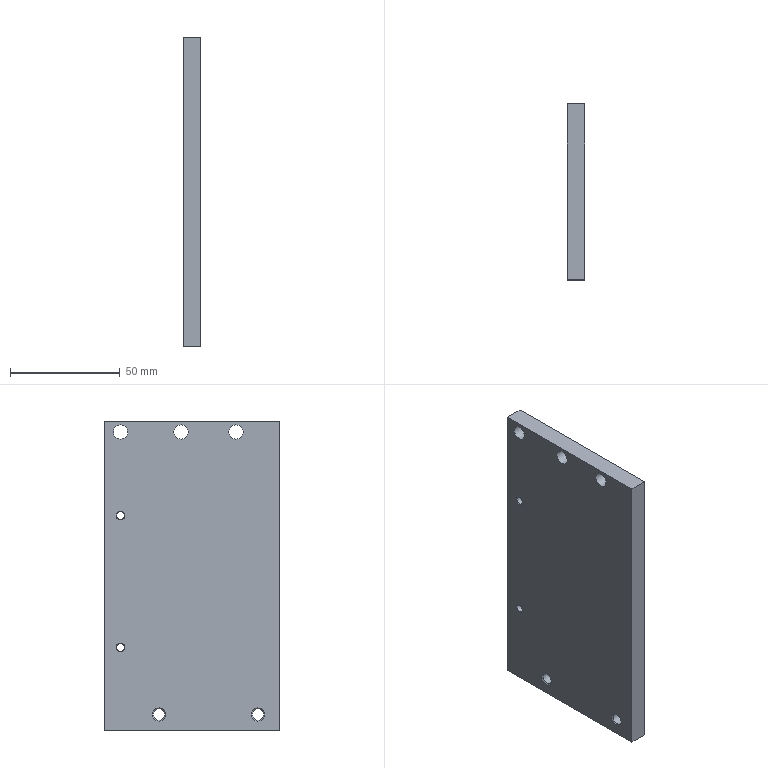Part | NX | features SIMPLE HOLE 7, DATUM_CSYS 5, SKETCH 4, SYMBOLIC_THREAD 4, HOLE PACKAGE 3, EXTRUDE 1 | 1 solid | 21 faces | box 8 x 80 x 141 mm | volume 88943 mm3 | cone 8 | cylinder 7 | plane 6 | commonest cylinder face diameters 6.5 x3 3.5 x2 5.2 x2
STEP:
#1=CARTESIAN_POINT('',(0.,-40.,70.5));
#2=VERTEX_POINT('',#1);
#3=CARTESIAN_POINT('',(0.,-40.,-70.5));
#4=VERTEX_POINT('',#3);
#5=CARTESIAN_POINT('',(0.,-40.,70.5));
#6=DIRECTION('',(0.,0.,-1.));
#7=VECTOR('',#6,1000.);
#8=LINE('',#5,#7);
#9=EDGE_CURVE('',#2,#4,#8,.T.);
#10=ORIENTED_EDGE('',*,*,#9,.T.);
#11=CARTESIAN_POINT('',(8.,-40.,-70.5));
#12=VERTEX_POINT('',#11);
#13=CARTESIAN_POINT('',(8.,-40.,-70.5));
#14=DIRECTION('',(-1.,0.,0.));
#15=VECTOR('',#14,1000.);
#16=LINE('',#13,#15);
#17=EDGE_CURVE('',#12,#4,#16,.T.);
#18=ORIENTED_EDGE('',*,*,#17,.F.);
#19=CARTESIAN_POINT('',(8.,-40.,70.5));
#20=VERTEX_POINT('',#19);
#21=CARTESIAN_POINT('',(8.,-40.,70.5));
#22=DIRECTION('',(0.,0.,-1.));
#23=VECTOR('',#22,1000.);
#24=LINE('',#21,#23);
#25=EDGE_CURVE('',#20,#12,#24,.T.);
#26=ORIENTED_EDGE('',*,*,#25,.F.);
#27=CARTESIAN_POINT('',(8.,-40.,70.5));
#28=DIRECTION('',(-1.,0.,0.));
#29=VECTOR('',#28,1000.);
#30=LINE('',#27,#29);
#31=EDGE_CURVE('',#20,#2,#30,.T.);
#32=ORIENTED_EDGE('',*,*,#31,.T.);
#33=EDGE_LOOP('',(#10,#18,#26,#32));
#34=FACE_BOUND('',#33,.T.);
#35=CARTESIAN_POINT('',(8.,-40.,70.5));
#36=DIRECTION('',(0.,1.,0.));
#37=DIRECTION('',(0.,0.,1.));
#38=AXIS2_PLACEMENT_3D('',#35,#36,#37);
#39=PLANE('',#38);
#40=ADVANCED_FACE('',(#34),#39,.F.);
#41=CARTESIAN_POINT('',(0.,40.,-70.5));
#42=VERTEX_POINT('',#41);
#43=CARTESIAN_POINT('',(0.,-40.,-70.5));
#44=DIRECTION('',(0.,1.,0.));
#45=VECTOR('',#44,1000.);
#46=LINE('',#43,#45);
#47=EDGE_CURVE('',#4,#42,#46,.T.);
#48=ORIENTED_EDGE('',*,*,#47,.T.);
#49=CARTESIAN_POINT('',(8.,40.,-70.5));
#50=VERTEX_POINT('',#49);
#51=CARTESIAN_POINT('',(8.,40.,-70.5));
#52=DIRECTION('',(-1.,0.,0.));
#53=VECTOR('',#52,1000.);
#54=LINE('',#51,#53);
#55=EDGE_CURVE('',#50,#42,#54,.T.);
#56=ORIENTED_EDGE('',*,*,#55,.F.);
#57=CARTESIAN_POINT('',(8.,-40.,-70.5));
#58=DIRECTION('',(0.,1.,0.));
#59=VECTOR('',#58,1000.);
#60=LINE('',#57,#59);
#61=EDGE_CURVE('',#12,#50,#60,.T.);
#62=ORIENTED_EDGE('',*,*,#61,.F.);
#63=ORIENTED_EDGE('',*,*,#17,.T.);
#64=EDGE_LOOP('',(#48,#56,#62,#63));
#65=FACE_BOUND('',#64,.T.);
#66=CARTESIAN_POINT('',(8.,-40.,-70.5));
#67=DIRECTION('',(0.,0.,1.));
#68=DIRECTION('',(1.,0.,0.));
#69=AXIS2_PLACEMENT_3D('',#66,#67,#68);
#70=PLANE('',#69);
#71=ADVANCED_FACE('',(#65),#70,.F.);
#72=CARTESIAN_POINT('',(0.,40.,70.5));
#73=VERTEX_POINT('',#72);
#74=CARTESIAN_POINT('',(0.,40.,-70.5));
#75=DIRECTION('',(0.,0.,1.));
#76=VECTOR('',#75,1000.);
#77=LINE('',#74,#76);
#78=EDGE_CURVE('',#42,#73,#77,.T.);
#79=ORIENTED_EDGE('',*,*,#78,.T.);
#80=CARTESIAN_POINT('',(8.,40.,70.5));
#81=VERTEX_POINT('',#80);
#82=CARTESIAN_POINT('',(8.,40.,70.5));
#83=DIRECTION('',(-1.,0.,0.));
#84=VECTOR('',#83,1000.);
#85=LINE('',#82,#84);
#86=EDGE_CURVE('',#81,#73,#85,.T.);
#87=ORIENTED_EDGE('',*,*,#86,.F.);
#88=CARTESIAN_POINT('',(8.,40.,-70.5));
#89=DIRECTION('',(0.,0.,1.));
#90=VECTOR('',#89,1000.);
#91=LINE('',#88,#90);
#92=EDGE_CURVE('',#50,#81,#91,.T.);
#93=ORIENTED_EDGE('',*,*,#92,.F.);
#94=ORIENTED_EDGE('',*,*,#55,.T.);
#95=EDGE_LOOP('',(#79,#87,#93,#94));
#96=FACE_BOUND('',#95,.T.);
#97=CARTESIAN_POINT('',(8.,40.,-70.5));
#98=DIRECTION('',(0.,-1.,0.));
#99=DIRECTION('',(0.,0.,-1.));
#100=AXIS2_PLACEMENT_3D('',#97,#98,#99);
#101=PLANE('',#100);
#102=ADVANCED_FACE('',(#96),#101,.F.);
#103=CARTESIAN_POINT('',(0.,40.,70.5));
#104=DIRECTION('',(0.,-1.,0.));
#105=VECTOR('',#104,1000.);
#106=LINE('',#103,#105);
#107=EDGE_CURVE('',#73,#2,#106,.T.);
#108=ORIENTED_EDGE('',*,*,#107,.T.);
#109=ORIENTED_EDGE('',*,*,#31,.F.);
#110=CARTESIAN_POINT('',(8.,40.,70.5));
#111=DIRECTION('',(0.,-1.,0.));
#112=VECTOR('',#111,1000.);
#113=LINE('',#110,#112);
#114=EDGE_CURVE('',#81,#20,#113,.T.);
#115=ORIENTED_EDGE('',*,*,#114,.F.);
#116=ORIENTED_EDGE('',*,*,#86,.T.);
#117=EDGE_LOOP('',(#108,#109,#115,#116));
#118=FACE_BOUND('',#117,.T.);
#119=CARTESIAN_POINT('',(8.,40.,70.5));
#120=DIRECTION('',(0.,0.,-1.));
#121=DIRECTION('',(-1.,0.,0.));
#122=AXIS2_PLACEMENT_3D('',#119,#120,#121);
#123=PLANE('',#122);
#124=ADVANCED_FACE('',(#118),#123,.F.);
#125=CARTESIAN_POINT('',(8.,32.5,62.25));
#126=VERTEX_POINT('',#125);
#127=CARTESIAN_POINT('',(8.,32.5,65.5));
#128=DIRECTION('',(1.,0.,0.));
#129=DIRECTION('',(0.,0.,-1.));
#130=AXIS2_PLACEMENT_3D('',#127,#128,#129);
#131=CIRCLE('',#130,3.25);
#132=EDGE_CURVE('',#126,#126,#131,.T.);
#133=ORIENTED_EDGE('',*,*,#132,.F.);
#134=EDGE_LOOP('',(#133));
#135=FACE_BOUND('',#134,.T.);
#136=CARTESIAN_POINT('',(8.,5.,62.25));
#137=VERTEX_POINT('',#136);
#138=CARTESIAN_POINT('',(8.,5.,65.5));
#139=DIRECTION('',(1.,0.,0.));
#140=DIRECTION('',(0.,0.,-1.));
#141=AXIS2_PLACEMENT_3D('',#138,#139,#140);
#142=CIRCLE('',#141,3.25);
#143=EDGE_CURVE('',#137,#137,#142,.T.);
#144=ORIENTED_EDGE('',*,*,#143,.F.);
#145=EDGE_LOOP('',(#144));
#146=FACE_BOUND('',#145,.T.);
#147=CARTESIAN_POINT('',(8.,-20.,62.25));
#148=VERTEX_POINT('',#147);
#149=CARTESIAN_POINT('',(8.,-20.,65.5));
#150=DIRECTION('',(1.,0.,0.));
#151=DIRECTION('',(0.,0.,-1.));
#152=AXIS2_PLACEMENT_3D('',#149,#150,#151);
#153=CIRCLE('',#152,3.25);
#154=EDGE_CURVE('',#148,#148,#153,.T.);
#155=ORIENTED_EDGE('',*,*,#154,.F.);
#156=EDGE_LOOP('',(#155));
#157=FACE_BOUND('',#156,.T.);
#158=CARTESIAN_POINT('',(8.,15.,-66.));
#159=VERTEX_POINT('',#158);
#160=CARTESIAN_POINT('',(8.,15.,-63.));
#161=DIRECTION('',(1.,0.,0.));
#162=DIRECTION('',(0.,0.,-1.));
#163=AXIS2_PLACEMENT_3D('',#160,#161,#162);
#164=CIRCLE('',#163,3.);
#165=EDGE_CURVE('',#159,#159,#164,.F.);
#166=ORIENTED_EDGE('',*,*,#165,.T.);
#167=EDGE_LOOP('',(#166));
#168=FACE_BOUND('',#167,.T.);
#169=CARTESIAN_POINT('',(8.,-30.,-66.));
#170=VERTEX_POINT('',#169);
#171=CARTESIAN_POINT('',(8.,-30.,-63.));
#172=DIRECTION('',(1.,0.,0.));
#173=DIRECTION('',(0.,0.,-1.));
#174=AXIS2_PLACEMENT_3D('',#171,#172,#173);
#175=CIRCLE('',#174,3.);
#176=EDGE_CURVE('',#170,#170,#175,.F.);
#177=ORIENTED_EDGE('',*,*,#176,.T.);
#178=EDGE_LOOP('',(#177));
#179=FACE_BOUND('',#178,.T.);
#180=CARTESIAN_POINT('',(8.,32.5,25.5));
#181=VERTEX_POINT('',#180);
#182=CARTESIAN_POINT('',(8.,32.5,27.5));
#183=DIRECTION('',(1.,0.,0.));
#184=DIRECTION('',(0.,0.,-1.));
#185=AXIS2_PLACEMENT_3D('',#182,#183,#184);
#186=CIRCLE('',#185,2.);
#187=EDGE_CURVE('',#181,#181,#186,.F.);
#188=ORIENTED_EDGE('',*,*,#187,.T.);
#189=EDGE_LOOP('',(#188));
#190=FACE_BOUND('',#189,.T.);
#191=CARTESIAN_POINT('',(8.,32.5,-34.5));
#192=VERTEX_POINT('',#191);
#193=CARTESIAN_POINT('',(8.,32.5,-32.5));
#194=DIRECTION('',(1.,0.,0.));
#195=DIRECTION('',(0.,0.,-1.));
#196=AXIS2_PLACEMENT_3D('',#193,#194,#195);
#197=CIRCLE('',#196,2.);
#198=EDGE_CURVE('',#192,#192,#197,.F.);
#199=ORIENTED_EDGE('',*,*,#198,.T.);
#200=EDGE_LOOP('',(#199));
#201=FACE_BOUND('',#200,.T.);
#202=ORIENTED_EDGE('',*,*,#25,.T.);
#203=ORIENTED_EDGE('',*,*,#61,.T.);
#204=ORIENTED_EDGE('',*,*,#92,.T.);
#205=ORIENTED_EDGE('',*,*,#114,.T.);
#206=EDGE_LOOP('',(#202,#203,#204,#205));
#207=FACE_BOUND('',#206,.T.);
#208=CARTESIAN_POINT('',(8.,0.,0.));
#209=DIRECTION('',(1.,0.,0.));
#210=DIRECTION('',(0.,0.,-1.));
#211=AXIS2_PLACEMENT_3D('',#208,#209,#210);
#212=PLANE('',#211);
#213=ADVANCED_FACE('',(#135,#146,#157,#168,#179,#190,#201,#207),#212,.T.);
#214=CARTESIAN_POINT('',(0.,32.5,62.25));
#215=VERTEX_POINT('',#214);
#216=CARTESIAN_POINT('',(0.,32.5,65.5));
#217=DIRECTION('',(1.,0.,0.));
#218=DIRECTION('',(0.,0.,-1.));
#219=AXIS2_PLACEMENT_3D('',#216,#217,#218);
#220=CIRCLE('',#219,3.25);
#221=EDGE_CURVE('',#215,#215,#220,.T.);
#222=ORIENTED_EDGE('',*,*,#221,.T.);
#223=EDGE_LOOP('',(#222));
#224=FACE_BOUND('',#223,.T.);
#225=CARTESIAN_POINT('',(0.,5.,62.25));
#226=VERTEX_POINT('',#225);
#227=CARTESIAN_POINT('',(0.,5.,65.5));
#228=DIRECTION('',(1.,0.,0.));
#229=DIRECTION('',(0.,0.,-1.));
#230=AXIS2_PLACEMENT_3D('',#227,#228,#229);
#231=CIRCLE('',#230,3.25);
#232=EDGE_CURVE('',#226,#226,#231,.T.);
#233=ORIENTED_EDGE('',*,*,#232,.T.);
#234=EDGE_LOOP('',(#233));
#235=FACE_BOUND('',#234,.T.);
#236=CARTESIAN_POINT('',(0.,-20.,62.25));
#237=VERTEX_POINT('',#236);
#238=CARTESIAN_POINT('',(0.,-20.,65.5));
#239=DIRECTION('',(1.,0.,0.));
#240=DIRECTION('',(0.,0.,-1.));
#241=AXIS2_PLACEMENT_3D('',#238,#239,#240);
#242=CIRCLE('',#241,3.25);
#243=EDGE_CURVE('',#237,#237,#242,.T.);
#244=ORIENTED_EDGE('',*,*,#243,.T.);
#245=EDGE_LOOP('',(#244));
#246=FACE_BOUND('',#245,.T.);
#247=CARTESIAN_POINT('',(0.,15.,-66.));
#248=VERTEX_POINT('',#247);
#249=CARTESIAN_POINT('',(0.,15.,-63.));
#250=DIRECTION('',(1.,0.,0.));
#251=DIRECTION('',(0.,0.,-1.));
#252=AXIS2_PLACEMENT_3D('',#249,#250,#251);
#253=CIRCLE('',#252,3.);
#254=EDGE_CURVE('',#248,#248,#253,.T.);
#255=ORIENTED_EDGE('',*,*,#254,.T.);
#256=EDGE_LOOP('',(#255));
#257=FACE_BOUND('',#256,.T.);
#258=CARTESIAN_POINT('',(0.,-30.,-66.));
#259=VERTEX_POINT('',#258);
#260=CARTESIAN_POINT('',(0.,-30.,-63.));
#261=DIRECTION('',(1.,0.,0.));
#262=DIRECTION('',(0.,0.,-1.));
#263=AXIS2_PLACEMENT_3D('',#260,#261,#262);
#264=CIRCLE('',#263,3.);
#265=EDGE_CURVE('',#259,#259,#264,.T.);
#266=ORIENTED_EDGE('',*,*,#265,.T.);
#267=EDGE_LOOP('',(#266));
#268=FACE_BOUND('',#267,.T.);
#269=CARTESIAN_POINT('',(0.,32.5,25.5));
#270=VERTEX_POINT('',#269);
#271=CARTESIAN_POINT('',(0.,32.5,27.5));
#272=DIRECTION('',(1.,0.,0.));
#273=DIRECTION('',(0.,0.,-1.));
#274=AXIS2_PLACEMENT_3D('',#271,#272,#273);
#275=CIRCLE('',#274,2.);
#276=EDGE_CURVE('',#270,#270,#275,.T.);
#277=ORIENTED_EDGE('',*,*,#276,.T.);
#278=EDGE_LOOP('',(#277));
#279=FACE_BOUND('',#278,.T.);
#280=CARTESIAN_POINT('',(0.,32.5,-34.5));
#281=VERTEX_POINT('',#280);
#282=CARTESIAN_POINT('',(0.,32.5,-32.5));
#283=DIRECTION('',(1.,0.,0.));
#284=DIRECTION('',(0.,0.,-1.));
#285=AXIS2_PLACEMENT_3D('',#282,#283,#284);
#286=CIRCLE('',#285,2.);
#287=EDGE_CURVE('',#281,#281,#286,.T.);
#288=ORIENTED_EDGE('',*,*,#287,.T.);
#289=EDGE_LOOP('',(#288));
#290=FACE_BOUND('',#289,.T.);
#291=ORIENTED_EDGE('',*,*,#9,.F.);
#292=ORIENTED_EDGE('',*,*,#107,.F.);
#293=ORIENTED_EDGE('',*,*,#78,.F.);
#294=ORIENTED_EDGE('',*,*,#47,.F.);
#295=EDGE_LOOP('',(#291,#292,#293,#294));
#296=FACE_BOUND('',#295,.T.);
#297=CARTESIAN_POINT('',(0.,0.,0.));
#298=DIRECTION('',(1.,0.,0.));
#299=DIRECTION('',(0.,0.,-1.));
#300=AXIS2_PLACEMENT_3D('',#297,#298,#299);
#301=PLANE('',#300);
#302=ADVANCED_FACE('',(#224,#235,#246,#257,#268,#279,#290,#296),#301,.F.);
#303=CARTESIAN_POINT('',(0.25,32.5,-34.25));
#304=VERTEX_POINT('',#303);
#305=CARTESIAN_POINT('',(0.25,32.5,-32.5));
#306=DIRECTION('',(1.,0.,0.));
#307=DIRECTION('',(0.,0.,-1.));
#308=AXIS2_PLACEMENT_3D('',#305,#306,#307);
#309=CIRCLE('',#308,1.75);
#310=EDGE_CURVE('',#304,#304,#309,.F.);
#311=ORIENTED_EDGE('',*,*,#310,.T.);
#312=EDGE_LOOP('',(#311));
#313=FACE_BOUND('',#312,.T.);
#314=CARTESIAN_POINT('',(7.75,32.5,-34.25));
#315=VERTEX_POINT('',#314);
#316=CARTESIAN_POINT('',(7.75,32.5,-32.5));
#317=DIRECTION('',(1.,0.,0.));
#318=DIRECTION('',(0.,0.,-1.));
#319=AXIS2_PLACEMENT_3D('',#316,#317,#318);
#320=CIRCLE('',#319,1.75);
#321=EDGE_CURVE('',#315,#315,#320,.T.);
#322=ORIENTED_EDGE('',*,*,#321,.T.);
#323=EDGE_LOOP('',(#322));
#324=FACE_BOUND('',#323,.T.);
#325=CARTESIAN_POINT('',(8.,32.5,-32.5));
#326=DIRECTION('',(-1.,0.,0.));
#327=DIRECTION('',(0.,0.,1.));
#328=AXIS2_PLACEMENT_3D('',#325,#326,#327);
#329=CYLINDRICAL_SURFACE('',#328,1.75);
#330=ADVANCED_FACE('',(#313,#324),#329,.F.);
#331=ORIENTED_EDGE('',*,*,#321,.F.);
#332=EDGE_LOOP('',(#331));
#333=FACE_BOUND('',#332,.T.);
#334=ORIENTED_EDGE('',*,*,#198,.F.);
#335=EDGE_LOOP('',(#334));
#336=FACE_BOUND('',#335,.T.);
#337=CARTESIAN_POINT('',(8.,32.5,-32.5));
#338=DIRECTION('',(1.,0.,0.));
#339=DIRECTION('',(0.,0.,-1.));
#340=AXIS2_PLACEMENT_3D('',#337,#338,#339);
#341=CONICAL_SURFACE('',#340,2.,0.7854);
#342=ADVANCED_FACE('',(#333,#336),#341,.F.);
#343=ORIENTED_EDGE('',*,*,#310,.F.);
#344=EDGE_LOOP('',(#343));
#345=FACE_BOUND('',#344,.T.);
#346=ORIENTED_EDGE('',*,*,#287,.F.);
#347=EDGE_LOOP('',(#346));
#348=FACE_BOUND('',#347,.T.);
#349=CARTESIAN_POINT('',(0.,32.5,-32.5));
#350=DIRECTION('',(-1.,0.,0.));
#351=DIRECTION('',(0.,0.,1.));
#352=AXIS2_PLACEMENT_3D('',#349,#350,#351);
#353=CONICAL_SURFACE('',#352,2.,0.7854);
#354=ADVANCED_FACE('',(#345,#348),#353,.F.);
#355=CARTESIAN_POINT('',(0.25,32.5,25.75));
#356=VERTEX_POINT('',#355);
#357=CARTESIAN_POINT('',(0.25,32.5,27.5));
#358=DIRECTION('',(1.,0.,0.));
#359=DIRECTION('',(0.,0.,-1.));
#360=AXIS2_PLACEMENT_3D('',#357,#358,#359);
#361=CIRCLE('',#360,1.75);
#362=EDGE_CURVE('',#356,#356,#361,.F.);
#363=ORIENTED_EDGE('',*,*,#362,.T.);
#364=EDGE_LOOP('',(#363));
#365=FACE_BOUND('',#364,.T.);
#366=CARTESIAN_POINT('',(7.75,32.5,25.75));
#367=VERTEX_POINT('',#366);
#368=CARTESIAN_POINT('',(7.75,32.5,27.5));
#369=DIRECTION('',(1.,0.,0.));
#370=DIRECTION('',(0.,0.,-1.));
#371=AXIS2_PLACEMENT_3D('',#368,#369,#370);
#372=CIRCLE('',#371,1.75);
#373=EDGE_CURVE('',#367,#367,#372,.T.);
#374=ORIENTED_EDGE('',*,*,#373,.T.);
#375=EDGE_LOOP('',(#374));
#376=FACE_BOUND('',#375,.T.);
#377=CARTESIAN_POINT('',(8.,32.5,27.5));
#378=DIRECTION('',(-1.,0.,0.));
#379=DIRECTION('',(0.,0.,1.));
#380=AXIS2_PLACEMENT_3D('',#377,#378,#379);
#381=CYLINDRICAL_SURFACE('',#380,1.75);
#382=ADVANCED_FACE('',(#365,#376),#381,.F.);
#383=ORIENTED_EDGE('',*,*,#373,.F.);
#384=EDGE_LOOP('',(#383));
#385=FACE_BOUND('',#384,.T.);
#386=ORIENTED_EDGE('',*,*,#187,.F.);
#387=EDGE_LOOP('',(#386));
#388=FACE_BOUND('',#387,.T.);
#389=CARTESIAN_POINT('',(8.,32.5,27.5));
#390=DIRECTION('',(1.,0.,0.));
#391=DIRECTION('',(0.,0.,-1.));
#392=AXIS2_PLACEMENT_3D('',#389,#390,#391);
#393=CONICAL_SURFACE('',#392,2.,0.7854);
#394=ADVANCED_FACE('',(#385,#388),#393,.F.);
#395=ORIENTED_EDGE('',*,*,#362,.F.);
#396=EDGE_LOOP('',(#395));
#397=FACE_BOUND('',#396,.T.);
#398=ORIENTED_EDGE('',*,*,#276,.F.);
#399=EDGE_LOOP('',(#398));
#400=FACE_BOUND('',#399,.T.);
#401=CARTESIAN_POINT('',(0.,32.5,27.5));
#402=DIRECTION('',(-1.,0.,0.));
#403=DIRECTION('',(0.,0.,1.));
#404=AXIS2_PLACEMENT_3D('',#401,#402,#403);
#405=CONICAL_SURFACE('',#404,2.,0.7854);
#406=ADVANCED_FACE('',(#397,#400),#405,.F.);
#407=CARTESIAN_POINT('',(0.4,-30.,-65.6));
#408=VERTEX_POINT('',#407);
#409=CARTESIAN_POINT('',(0.4,-30.,-63.));
#410=DIRECTION('',(1.,0.,0.));
#411=DIRECTION('',(0.,0.,-1.));
#412=AXIS2_PLACEMENT_3D('',#409,#410,#411);
#413=CIRCLE('',#412,2.6);
#414=EDGE_CURVE('',#408,#408,#413,.F.);
#415=ORIENTED_EDGE('',*,*,#414,.T.);
#416=EDGE_LOOP('',(#415));
#417=FACE_BOUND('',#416,.T.);
#418=CARTESIAN_POINT('',(7.6,-30.,-65.6));
#419=VERTEX_POINT('',#418);
#420=CARTESIAN_POINT('',(7.6,-30.,-63.));
#421=DIRECTION('',(1.,0.,0.));
#422=DIRECTION('',(0.,0.,-1.));
#423=AXIS2_PLACEMENT_3D('',#420,#421,#422);
#424=CIRCLE('',#423,2.6);
#425=EDGE_CURVE('',#419,#419,#424,.T.);
#426=ORIENTED_EDGE('',*,*,#425,.T.);
#427=EDGE_LOOP('',(#426));
#428=FACE_BOUND('',#427,.T.);
#429=CARTESIAN_POINT('',(8.,-30.,-63.));
#430=DIRECTION('',(-1.,0.,0.));
#431=DIRECTION('',(0.,0.,1.));
#432=AXIS2_PLACEMENT_3D('',#429,#430,#431);
#433=CYLINDRICAL_SURFACE('',#432,2.6);
#434=ADVANCED_FACE('',(#417,#428),#433,.F.);
#435=ORIENTED_EDGE('',*,*,#425,.F.);
#436=EDGE_LOOP('',(#435));
#437=FACE_BOUND('',#436,.T.);
#438=ORIENTED_EDGE('',*,*,#176,.F.);
#439=EDGE_LOOP('',(#438));
#440=FACE_BOUND('',#439,.T.);
#441=CARTESIAN_POINT('',(8.,-30.,-63.));
#442=DIRECTION('',(1.,0.,0.));
#443=DIRECTION('',(0.,0.,-1.));
#444=AXIS2_PLACEMENT_3D('',#441,#442,#443);
#445=CONICAL_SURFACE('',#444,3.,0.7854);
#446=ADVANCED_FACE('',(#437,#440),#445,.F.);
#447=ORIENTED_EDGE('',*,*,#414,.F.);
#448=EDGE_LOOP('',(#447));
#449=FACE_BOUND('',#448,.T.);
#450=ORIENTED_EDGE('',*,*,#265,.F.);
#451=EDGE_LOOP('',(#450));
#452=FACE_BOUND('',#451,.T.);
#453=CARTESIAN_POINT('',(0.,-30.,-63.));
#454=DIRECTION('',(-1.,0.,0.));
#455=DIRECTION('',(0.,0.,1.));
#456=AXIS2_PLACEMENT_3D('',#453,#454,#455);
#457=CONICAL_SURFACE('',#456,3.,0.7854);
#458=ADVANCED_FACE('',(#449,#452),#457,.F.);
#459=CARTESIAN_POINT('',(0.4,15.,-65.6));
#460=VERTEX_POINT('',#459);
#461=CARTESIAN_POINT('',(0.4,15.,-63.));
#462=DIRECTION('',(1.,0.,0.));
#463=DIRECTION('',(0.,0.,-1.));
#464=AXIS2_PLACEMENT_3D('',#461,#462,#463);
#465=CIRCLE('',#464,2.6);
#466=EDGE_CURVE('',#460,#460,#465,.F.);
#467=ORIENTED_EDGE('',*,*,#466,.T.);
#468=EDGE_LOOP('',(#467));
#469=FACE_BOUND('',#468,.T.);
#470=CARTESIAN_POINT('',(7.6,15.,-65.6));
#471=VERTEX_POINT('',#470);
#472=CARTESIAN_POINT('',(7.6,15.,-63.));
#473=DIRECTION('',(1.,0.,0.));
#474=DIRECTION('',(0.,0.,-1.));
#475=AXIS2_PLACEMENT_3D('',#472,#473,#474);
#476=CIRCLE('',#475,2.6);
#477=EDGE_CURVE('',#471,#471,#476,.T.);
#478=ORIENTED_EDGE('',*,*,#477,.T.);
#479=EDGE_LOOP('',(#478));
#480=FACE_BOUND('',#479,.T.);
#481=CARTESIAN_POINT('',(8.,15.,-63.));
#482=DIRECTION('',(-1.,0.,0.));
#483=DIRECTION('',(0.,0.,1.));
#484=AXIS2_PLACEMENT_3D('',#481,#482,#483);
#485=CYLINDRICAL_SURFACE('',#484,2.6);
#486=ADVANCED_FACE('',(#469,#480),#485,.F.);
#487=ORIENTED_EDGE('',*,*,#477,.F.);
#488=EDGE_LOOP('',(#487));
#489=FACE_BOUND('',#488,.T.);
#490=ORIENTED_EDGE('',*,*,#165,.F.);
#491=EDGE_LOOP('',(#490));
#492=FACE_BOUND('',#491,.T.);
#493=CARTESIAN_POINT('',(8.,15.,-63.));
#494=DIRECTION('',(1.,0.,0.));
#495=DIRECTION('',(0.,0.,-1.));
#496=AXIS2_PLACEMENT_3D('',#493,#494,#495);
#497=CONICAL_SURFACE('',#496,3.,0.7854);
#498=ADVANCED_FACE('',(#489,#492),#497,.F.);
#499=ORIENTED_EDGE('',*,*,#466,.F.);
#500=EDGE_LOOP('',(#499));
#501=FACE_BOUND('',#500,.T.);
#502=ORIENTED_EDGE('',*,*,#254,.F.);
#503=EDGE_LOOP('',(#502));
#504=FACE_BOUND('',#503,.T.);
#505=CARTESIAN_POINT('',(0.,15.,-63.));
#506=DIRECTION('',(-1.,0.,0.));
#507=DIRECTION('',(0.,0.,1.));
#508=AXIS2_PLACEMENT_3D('',#505,#506,#507);
#509=CONICAL_SURFACE('',#508,3.,0.7854);
#510=ADVANCED_FACE('',(#501,#504),#509,.F.);
#511=ORIENTED_EDGE('',*,*,#154,.T.);
#512=EDGE_LOOP('',(#511));
#513=FACE_BOUND('',#512,.T.);
#514=ORIENTED_EDGE('',*,*,#243,.F.);
#515=EDGE_LOOP('',(#514));
#516=FACE_BOUND('',#515,.T.);
#517=CARTESIAN_POINT('',(0.,-20.,65.5));
#518=DIRECTION('',(1.,0.,0.));
#519=DIRECTION('',(0.,0.,-1.));
#520=AXIS2_PLACEMENT_3D('',#517,#518,#519);
#521=CYLINDRICAL_SURFACE('',#520,3.25);
#522=ADVANCED_FACE('',(#513,#516),#521,.F.);
#523=ORIENTED_EDGE('',*,*,#143,.T.);
#524=EDGE_LOOP('',(#523));
#525=FACE_BOUND('',#524,.T.);
#526=ORIENTED_EDGE('',*,*,#232,.F.);
#527=EDGE_LOOP('',(#526));
#528=FACE_BOUND('',#527,.T.);
#529=CARTESIAN_POINT('',(0.,5.,65.5));
#530=DIRECTION('',(1.,0.,0.));
#531=DIRECTION('',(0.,0.,-1.));
#532=AXIS2_PLACEMENT_3D('',#529,#530,#531);
#533=CYLINDRICAL_SURFACE('',#532,3.25);
#534=ADVANCED_FACE('',(#525,#528),#533,.F.);
#535=ORIENTED_EDGE('',*,*,#132,.T.);
#536=EDGE_LOOP('',(#535));
#537=FACE_BOUND('',#536,.T.);
#538=ORIENTED_EDGE('',*,*,#221,.F.);
#539=EDGE_LOOP('',(#538));
#540=FACE_BOUND('',#539,.T.);
#541=CARTESIAN_POINT('',(0.,32.5,65.5));
#542=DIRECTION('',(1.,0.,0.));
#543=DIRECTION('',(0.,0.,-1.));
#544=AXIS2_PLACEMENT_3D('',#541,#542,#543);
#545=CYLINDRICAL_SURFACE('',#544,3.25);
#546=ADVANCED_FACE('',(#537,#540),#545,.F.);
#547=CLOSED_SHELL('',(#40,#71,#102,#124,#213,#302,#330,#342,#354,#382,#394,#406,#434,#446,#458,#486,#498,#510,#522,#534,#546));
#548=MANIFOLD_SOLID_BREP('',#547);
#549=(LENGTH_UNIT()NAMED_UNIT(*)SI_UNIT(.MILLI.,.METRE.));
#550=UNCERTAINTY_MEASURE_WITH_UNIT(LENGTH_MEASURE(0.00001),#549,'','');
#551=(NAMED_UNIT(*)PLANE_ANGLE_UNIT()SI_UNIT($,.RADIAN.));
#552=(NAMED_UNIT(*)SI_UNIT($,.STERADIAN.)SOLID_ANGLE_UNIT());
#553=(GEOMETRIC_REPRESENTATION_CONTEXT(3)GLOBAL_UNCERTAINTY_ASSIGNED_CONTEXT((#550))GLOBAL_UNIT_ASSIGNED_CONTEXT((#549,#551,#552))REPRESENTATION_CONTEXT('',''));
#554=ADVANCED_BREP_SHAPE_REPRESENTATION('',(#548),#553);